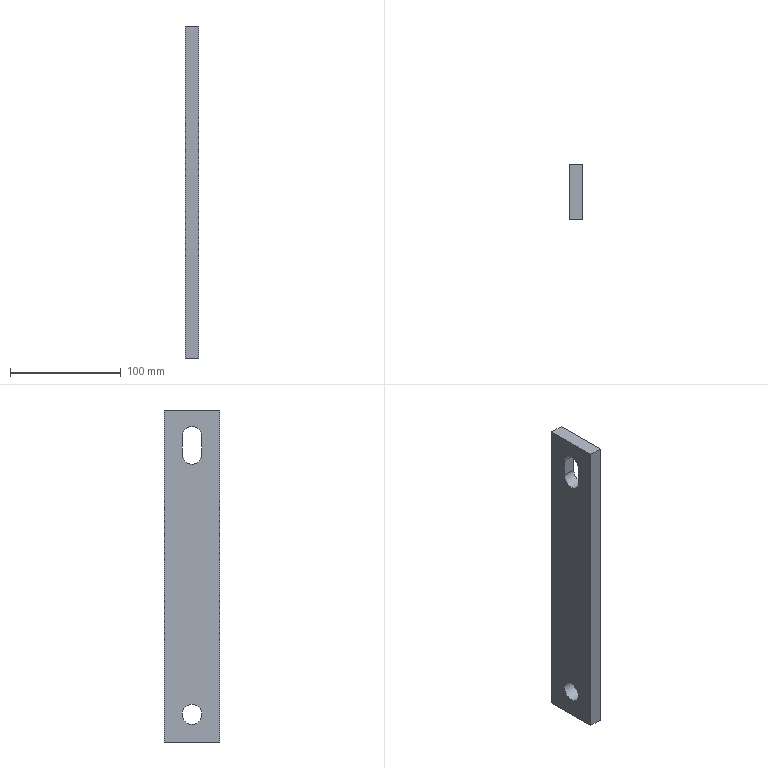Part | NX | features solid 2 | 1 solid | 11 faces | box 12 x 50 x 300 mm | volume 170437 mm3 | plane 8 | cylinder 3 | commonest cylinder face diameters 18 x3
STEP:
#1=CARTESIAN_POINT('',(1560.,-580.,-444.));
#2=VERTEX_POINT('',#1);
#3=CARTESIAN_POINT('',(1560.,-580.,-435.));
#4=DIRECTION('',(-1.,0.,0.));
#5=DIRECTION('',(0.,0.,-1.));
#6=AXIS2_PLACEMENT_3D('',#3,#4,#5);
#7=CIRCLE('',#6,9.);
#8=EDGE_CURVE('',#2,#2,#7,.F.);
#9=ORIENTED_EDGE('',*,*,#8,.T.);
#10=EDGE_LOOP('',(#9));
#11=FACE_BOUND('',#10,.T.);
#12=CARTESIAN_POINT('',(1560.,-605.,-460.));
#13=VERTEX_POINT('',#12);
#14=CARTESIAN_POINT('',(1560.,-555.,-460.));
#15=VERTEX_POINT('',#14);
#16=CARTESIAN_POINT('',(1560.,-600.,-460.));
#17=DIRECTION('',(0.,1.,0.));
#18=VECTOR('',#17,1000.);
#19=LINE('',#16,#18);
#20=EDGE_CURVE('',#13,#15,#19,.T.);
#21=ORIENTED_EDGE('',*,*,#20,.F.);
#22=CARTESIAN_POINT('',(1560.,-605.,-160.));
#23=VERTEX_POINT('',#22);
#24=CARTESIAN_POINT('',(1560.,-605.,-345.));
#25=DIRECTION('',(0.,0.,1.));
#26=VECTOR('',#25,1000.);
#27=LINE('',#24,#26);
#28=EDGE_CURVE('',#13,#23,#27,.T.);
#29=ORIENTED_EDGE('',*,*,#28,.T.);
#30=CARTESIAN_POINT('',(1560.,-555.,-160.));
#31=VERTEX_POINT('',#30);
#32=CARTESIAN_POINT('',(1560.,-600.,-160.));
#33=DIRECTION('',(0.,-1.,0.));
#34=VECTOR('',#33,1000.);
#35=LINE('',#32,#34);
#36=EDGE_CURVE('',#31,#23,#35,.T.);
#37=ORIENTED_EDGE('',*,*,#36,.F.);
#38=CARTESIAN_POINT('',(1560.,-555.,-345.));
#39=DIRECTION('',(0.,0.,1.));
#40=VECTOR('',#39,1000.);
#41=LINE('',#38,#40);
#42=EDGE_CURVE('',#15,#31,#41,.T.);
#43=ORIENTED_EDGE('',*,*,#42,.F.);
#44=EDGE_LOOP('',(#21,#29,#37,#43));
#45=FACE_BOUND('',#44,.T.);
#46=CARTESIAN_POINT('',(1560.,-571.,-200.));
#47=VERTEX_POINT('',#46);
#48=CARTESIAN_POINT('',(1560.,-571.,-184.));
#49=VERTEX_POINT('',#48);
#50=CARTESIAN_POINT('',(1560.,-571.,-352.));
#51=DIRECTION('',(0.,0.,1.));
#52=VECTOR('',#51,1000.);
#53=LINE('',#50,#52);
#54=EDGE_CURVE('',#47,#49,#53,.T.);
#55=ORIENTED_EDGE('',*,*,#54,.T.);
#56=CARTESIAN_POINT('',(1560.,-589.,-184.));
#57=VERTEX_POINT('',#56);
#58=CARTESIAN_POINT('',(1560.,-580.,-184.));
#59=DIRECTION('',(-1.,0.,0.));
#60=DIRECTION('',(0.,0.,-1.));
#61=AXIS2_PLACEMENT_3D('',#58,#59,#60);
#62=CIRCLE('',#61,9.);
#63=EDGE_CURVE('',#57,#49,#62,.T.);
#64=ORIENTED_EDGE('',*,*,#63,.F.);
#65=CARTESIAN_POINT('',(1560.,-589.,-200.));
#66=VERTEX_POINT('',#65);
#67=CARTESIAN_POINT('',(1560.,-589.,-352.));
#68=DIRECTION('',(0.,0.,1.));
#69=VECTOR('',#68,1000.);
#70=LINE('',#67,#69);
#71=EDGE_CURVE('',#66,#57,#70,.T.);
#72=ORIENTED_EDGE('',*,*,#71,.F.);
#73=CARTESIAN_POINT('',(1560.,-580.,-200.));
#74=DIRECTION('',(-1.,0.,0.));
#75=DIRECTION('',(0.,0.,-1.));
#76=AXIS2_PLACEMENT_3D('',#73,#74,#75);
#77=CIRCLE('',#76,9.);
#78=EDGE_CURVE('',#47,#66,#77,.T.);
#79=ORIENTED_EDGE('',*,*,#78,.F.);
#80=EDGE_LOOP('',(#55,#64,#72,#79));
#81=FACE_BOUND('',#80,.T.);
#82=CARTESIAN_POINT('',(1560.,-600.,-345.));
#83=DIRECTION('',(1.,0.,0.));
#84=DIRECTION('',(0.,0.,-1.));
#85=AXIS2_PLACEMENT_3D('',#82,#83,#84);
#86=PLANE('',#85);
#87=ADVANCED_FACE('',(#11,#45,#81),#86,.F.);
#88=CARTESIAN_POINT('',(1572.,-580.,-444.));
#89=VERTEX_POINT('',#88);
#90=CARTESIAN_POINT('',(1572.,-580.,-435.));
#91=DIRECTION('',(-1.,0.,0.));
#92=DIRECTION('',(0.,0.,-1.));
#93=AXIS2_PLACEMENT_3D('',#90,#91,#92);
#94=CIRCLE('',#93,9.);
#95=EDGE_CURVE('',#89,#89,#94,.T.);
#96=ORIENTED_EDGE('',*,*,#95,.T.);
#97=EDGE_LOOP('',(#96));
#98=FACE_BOUND('',#97,.T.);
#99=CARTESIAN_POINT('',(1572.,-605.,-460.));
#100=VERTEX_POINT('',#99);
#101=CARTESIAN_POINT('',(1572.,-555.,-460.));
#102=VERTEX_POINT('',#101);
#103=CARTESIAN_POINT('',(1572.,-600.,-460.));
#104=DIRECTION('',(0.,1.,0.));
#105=VECTOR('',#104,1000.);
#106=LINE('',#103,#105);
#107=EDGE_CURVE('',#100,#102,#106,.T.);
#108=ORIENTED_EDGE('',*,*,#107,.T.);
#109=CARTESIAN_POINT('',(1572.,-555.,-160.));
#110=VERTEX_POINT('',#109);
#111=CARTESIAN_POINT('',(1572.,-555.,-345.));
#112=DIRECTION('',(0.,0.,1.));
#113=VECTOR('',#112,1000.);
#114=LINE('',#111,#113);
#115=EDGE_CURVE('',#102,#110,#114,.T.);
#116=ORIENTED_EDGE('',*,*,#115,.T.);
#117=CARTESIAN_POINT('',(1572.,-605.,-160.));
#118=VERTEX_POINT('',#117);
#119=CARTESIAN_POINT('',(1572.,-600.,-160.));
#120=DIRECTION('',(0.,-1.,0.));
#121=VECTOR('',#120,1000.);
#122=LINE('',#119,#121);
#123=EDGE_CURVE('',#110,#118,#122,.T.);
#124=ORIENTED_EDGE('',*,*,#123,.T.);
#125=CARTESIAN_POINT('',(1572.,-605.,-345.));
#126=DIRECTION('',(0.,0.,1.));
#127=VECTOR('',#126,1000.);
#128=LINE('',#125,#127);
#129=EDGE_CURVE('',#100,#118,#128,.T.);
#130=ORIENTED_EDGE('',*,*,#129,.F.);
#131=EDGE_LOOP('',(#108,#116,#124,#130));
#132=FACE_BOUND('',#131,.T.);
#133=CARTESIAN_POINT('',(1572.,-589.,-200.));
#134=VERTEX_POINT('',#133);
#135=CARTESIAN_POINT('',(1572.,-571.,-200.));
#136=VERTEX_POINT('',#135);
#137=CARTESIAN_POINT('',(1572.,-580.,-200.));
#138=DIRECTION('',(1.,0.,0.));
#139=DIRECTION('',(0.,0.,1.));
#140=AXIS2_PLACEMENT_3D('',#137,#138,#139);
#141=CIRCLE('',#140,9.);
#142=EDGE_CURVE('',#134,#136,#141,.T.);
#143=ORIENTED_EDGE('',*,*,#142,.F.);
#144=CARTESIAN_POINT('',(1572.,-589.,-184.));
#145=VERTEX_POINT('',#144);
#146=CARTESIAN_POINT('',(1572.,-589.,15.));
#147=DIRECTION('',(0.,0.,1.));
#148=VECTOR('',#147,1000.);
#149=LINE('',#146,#148);
#150=EDGE_CURVE('',#134,#145,#149,.T.);
#151=ORIENTED_EDGE('',*,*,#150,.T.);
#152=CARTESIAN_POINT('',(1572.,-571.,-184.));
#153=VERTEX_POINT('',#152);
#154=CARTESIAN_POINT('',(1572.,-580.,-184.));
#155=DIRECTION('',(1.,0.,0.));
#156=DIRECTION('',(0.,0.,1.));
#157=AXIS2_PLACEMENT_3D('',#154,#155,#156);
#158=CIRCLE('',#157,9.);
#159=EDGE_CURVE('',#153,#145,#158,.T.);
#160=ORIENTED_EDGE('',*,*,#159,.F.);
#161=CARTESIAN_POINT('',(1572.,-571.,15.));
#162=DIRECTION('',(0.,0.,1.));
#163=VECTOR('',#162,1000.);
#164=LINE('',#161,#163);
#165=EDGE_CURVE('',#136,#153,#164,.T.);
#166=ORIENTED_EDGE('',*,*,#165,.F.);
#167=EDGE_LOOP('',(#143,#151,#160,#166));
#168=FACE_BOUND('',#167,.T.);
#169=CARTESIAN_POINT('',(1572.,-600.,-345.));
#170=DIRECTION('',(1.,0.,0.));
#171=DIRECTION('',(0.,0.,-1.));
#172=AXIS2_PLACEMENT_3D('',#169,#170,#171);
#173=PLANE('',#172);
#174=ADVANCED_FACE('',(#98,#132,#168),#173,.T.);
#175=ORIENTED_EDGE('',*,*,#78,.T.);
#176=CARTESIAN_POINT('',(1522.,-589.,-200.));
#177=DIRECTION('',(1.,0.,0.));
#178=VECTOR('',#177,1000.);
#179=LINE('',#176,#178);
#180=EDGE_CURVE('',#66,#134,#179,.T.);
#181=ORIENTED_EDGE('',*,*,#180,.T.);
#182=ORIENTED_EDGE('',*,*,#142,.T.);
#183=CARTESIAN_POINT('',(1522.,-571.,-200.));
#184=DIRECTION('',(1.,0.,0.));
#185=VECTOR('',#184,1000.);
#186=LINE('',#183,#185);
#187=EDGE_CURVE('',#47,#136,#186,.T.);
#188=ORIENTED_EDGE('',*,*,#187,.F.);
#189=EDGE_LOOP('',(#175,#181,#182,#188));
#190=FACE_BOUND('',#189,.T.);
#191=CARTESIAN_POINT('',(1572.,-580.,-200.));
#192=DIRECTION('',(-1.,0.,0.));
#193=DIRECTION('',(0.,0.,1.));
#194=AXIS2_PLACEMENT_3D('',#191,#192,#193);
#195=CYLINDRICAL_SURFACE('',#194,9.);
#196=ADVANCED_FACE('',(#190),#195,.F.);
#197=CARTESIAN_POINT('',(1522.,-571.,-184.));
#198=DIRECTION('',(1.,0.,0.));
#199=VECTOR('',#198,1000.);
#200=LINE('',#197,#199);
#201=EDGE_CURVE('',#49,#153,#200,.T.);
#202=ORIENTED_EDGE('',*,*,#201,.T.);
#203=ORIENTED_EDGE('',*,*,#159,.T.);
#204=CARTESIAN_POINT('',(1522.,-589.,-184.));
#205=DIRECTION('',(1.,0.,0.));
#206=VECTOR('',#205,1000.);
#207=LINE('',#204,#206);
#208=EDGE_CURVE('',#57,#145,#207,.T.);
#209=ORIENTED_EDGE('',*,*,#208,.F.);
#210=ORIENTED_EDGE('',*,*,#63,.T.);
#211=EDGE_LOOP('',(#202,#203,#209,#210));
#212=FACE_BOUND('',#211,.T.);
#213=CARTESIAN_POINT('',(1572.,-580.,-184.));
#214=DIRECTION('',(-1.,0.,0.));
#215=DIRECTION('',(0.,0.,1.));
#216=AXIS2_PLACEMENT_3D('',#213,#214,#215);
#217=CYLINDRICAL_SURFACE('',#216,9.);
#218=ADVANCED_FACE('',(#212),#217,.F.);
#219=ORIENTED_EDGE('',*,*,#107,.F.);
#220=CARTESIAN_POINT('',(1560.,-605.,-460.));
#221=DIRECTION('',(1.,0.,0.));
#222=VECTOR('',#221,1000.);
#223=LINE('',#220,#222);
#224=EDGE_CURVE('',#13,#100,#223,.T.);
#225=ORIENTED_EDGE('',*,*,#224,.F.);
#226=ORIENTED_EDGE('',*,*,#20,.T.);
#227=CARTESIAN_POINT('',(1560.,-555.,-460.));
#228=DIRECTION('',(1.,0.,0.));
#229=VECTOR('',#228,1000.);
#230=LINE('',#227,#229);
#231=EDGE_CURVE('',#15,#102,#230,.T.);
#232=ORIENTED_EDGE('',*,*,#231,.T.);
#233=EDGE_LOOP('',(#219,#225,#226,#232));
#234=FACE_BOUND('',#233,.T.);
#235=CARTESIAN_POINT('',(1560.,-600.,-460.));
#236=DIRECTION('',(0.,0.,-1.));
#237=DIRECTION('',(1.,0.,0.));
#238=AXIS2_PLACEMENT_3D('',#235,#236,#237);
#239=PLANE('',#238);
#240=ADVANCED_FACE('',(#234),#239,.T.);
#241=ORIENTED_EDGE('',*,*,#115,.F.);
#242=ORIENTED_EDGE('',*,*,#231,.F.);
#243=ORIENTED_EDGE('',*,*,#42,.T.);
#244=CARTESIAN_POINT('',(1560.,-555.,-160.));
#245=DIRECTION('',(1.,0.,0.));
#246=VECTOR('',#245,1000.);
#247=LINE('',#244,#246);
#248=EDGE_CURVE('',#31,#110,#247,.T.);
#249=ORIENTED_EDGE('',*,*,#248,.T.);
#250=EDGE_LOOP('',(#241,#242,#243,#249));
#251=FACE_BOUND('',#250,.T.);
#252=CARTESIAN_POINT('',(1560.,-555.,-345.));
#253=DIRECTION('',(0.,1.,0.));
#254=DIRECTION('',(0.,0.,-1.));
#255=AXIS2_PLACEMENT_3D('',#252,#253,#254);
#256=PLANE('',#255);
#257=ADVANCED_FACE('',(#251),#256,.T.);
#258=ORIENTED_EDGE('',*,*,#123,.F.);
#259=ORIENTED_EDGE('',*,*,#248,.F.);
#260=ORIENTED_EDGE('',*,*,#36,.T.);
#261=CARTESIAN_POINT('',(1560.,-605.,-160.));
#262=DIRECTION('',(1.,0.,0.));
#263=VECTOR('',#262,1000.);
#264=LINE('',#261,#263);
#265=EDGE_CURVE('',#23,#118,#264,.T.);
#266=ORIENTED_EDGE('',*,*,#265,.T.);
#267=EDGE_LOOP('',(#258,#259,#260,#266));
#268=FACE_BOUND('',#267,.T.);
#269=CARTESIAN_POINT('',(1530.,-600.,-160.));
#270=DIRECTION('',(0.,0.,1.));
#271=DIRECTION('',(1.,0.,0.));
#272=AXIS2_PLACEMENT_3D('',#269,#270,#271);
#273=PLANE('',#272);
#274=ADVANCED_FACE('',(#268),#273,.T.);
#275=ORIENTED_EDGE('',*,*,#129,.T.);
#276=ORIENTED_EDGE('',*,*,#265,.F.);
#277=ORIENTED_EDGE('',*,*,#28,.F.);
#278=ORIENTED_EDGE('',*,*,#224,.T.);
#279=EDGE_LOOP('',(#275,#276,#277,#278));
#280=FACE_BOUND('',#279,.T.);
#281=CARTESIAN_POINT('',(1560.,-605.,-345.));
#282=DIRECTION('',(0.,1.,0.));
#283=DIRECTION('',(0.,0.,-1.));
#284=AXIS2_PLACEMENT_3D('',#281,#282,#283);
#285=PLANE('',#284);
#286=ADVANCED_FACE('',(#280),#285,.F.);
#287=ORIENTED_EDGE('',*,*,#95,.F.);
#288=EDGE_LOOP('',(#287));
#289=FACE_BOUND('',#288,.T.);
#290=ORIENTED_EDGE('',*,*,#8,.F.);
#291=EDGE_LOOP('',(#290));
#292=FACE_BOUND('',#291,.T.);
#293=CARTESIAN_POINT('',(1569.,-580.,-435.));
#294=DIRECTION('',(-1.,0.,0.));
#295=DIRECTION('',(0.,0.,-1.));
#296=AXIS2_PLACEMENT_3D('',#293,#294,#295);
#297=CYLINDRICAL_SURFACE('',#296,9.);
#298=ADVANCED_FACE('',(#289,#292),#297,.F.);
#299=ORIENTED_EDGE('',*,*,#71,.T.);
#300=ORIENTED_EDGE('',*,*,#208,.T.);
#301=ORIENTED_EDGE('',*,*,#150,.F.);
#302=ORIENTED_EDGE('',*,*,#180,.F.);
#303=EDGE_LOOP('',(#299,#300,#301,#302));
#304=FACE_BOUND('',#303,.T.);
#305=CARTESIAN_POINT('',(1522.,-589.,15.));
#306=DIRECTION('',(0.,-1.,0.));
#307=DIRECTION('',(0.,0.,1.));
#308=AXIS2_PLACEMENT_3D('',#305,#306,#307);
#309=PLANE('',#308);
#310=ADVANCED_FACE('',(#304),#309,.F.);
#311=ORIENTED_EDGE('',*,*,#54,.F.);
#312=ORIENTED_EDGE('',*,*,#187,.T.);
#313=ORIENTED_EDGE('',*,*,#165,.T.);
#314=ORIENTED_EDGE('',*,*,#201,.F.);
#315=EDGE_LOOP('',(#311,#312,#313,#314));
#316=FACE_BOUND('',#315,.T.);
#317=CARTESIAN_POINT('',(1522.,-571.,15.));
#318=DIRECTION('',(0.,-1.,0.));
#319=DIRECTION('',(0.,0.,1.));
#320=AXIS2_PLACEMENT_3D('',#317,#318,#319);
#321=PLANE('',#320);
#322=ADVANCED_FACE('',(#316),#321,.T.);
#323=CLOSED_SHELL('',(#87,#174,#196,#218,#240,#257,#274,#286,#298,#310,#322));
#324=MANIFOLD_SOLID_BREP('',#323);
#325=(LENGTH_UNIT()NAMED_UNIT(*)SI_UNIT(.MILLI.,.METRE.));
#326=UNCERTAINTY_MEASURE_WITH_UNIT(LENGTH_MEASURE(0.00001),#325,'','');
#327=(NAMED_UNIT(*)PLANE_ANGLE_UNIT()SI_UNIT($,.RADIAN.));
#328=(NAMED_UNIT(*)SI_UNIT($,.STERADIAN.)SOLID_ANGLE_UNIT());
#329=(GEOMETRIC_REPRESENTATION_CONTEXT(3)GLOBAL_UNCERTAINTY_ASSIGNED_CONTEXT((#326))GLOBAL_UNIT_ASSIGNED_CONTEXT((#325,#327,#328))REPRESENTATION_CONTEXT('',''));
#330=ADVANCED_BREP_SHAPE_REPRESENTATION('',(#324),#329);